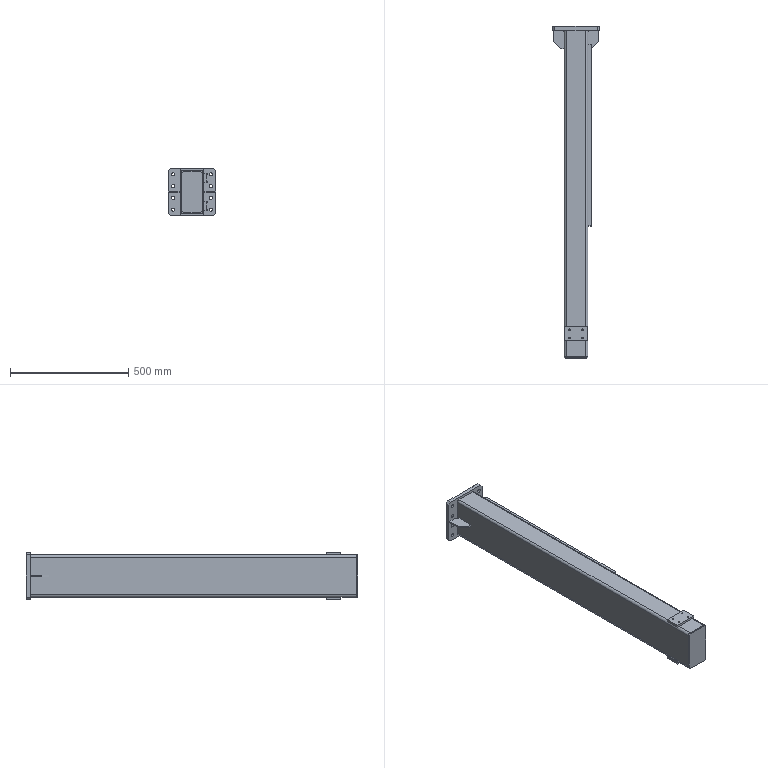Part | STEP file | YCD14007A-08.02.01 Slide | 3 solids | 186 faces | box 200 x 1406 x 200 mm | volume 5203563 mm3 | cylinder 102 | plane 84 | commonest cylinder face diameters 6.8 x64 13.5 x16 20 x12 26 x4 1 x2 16 x2